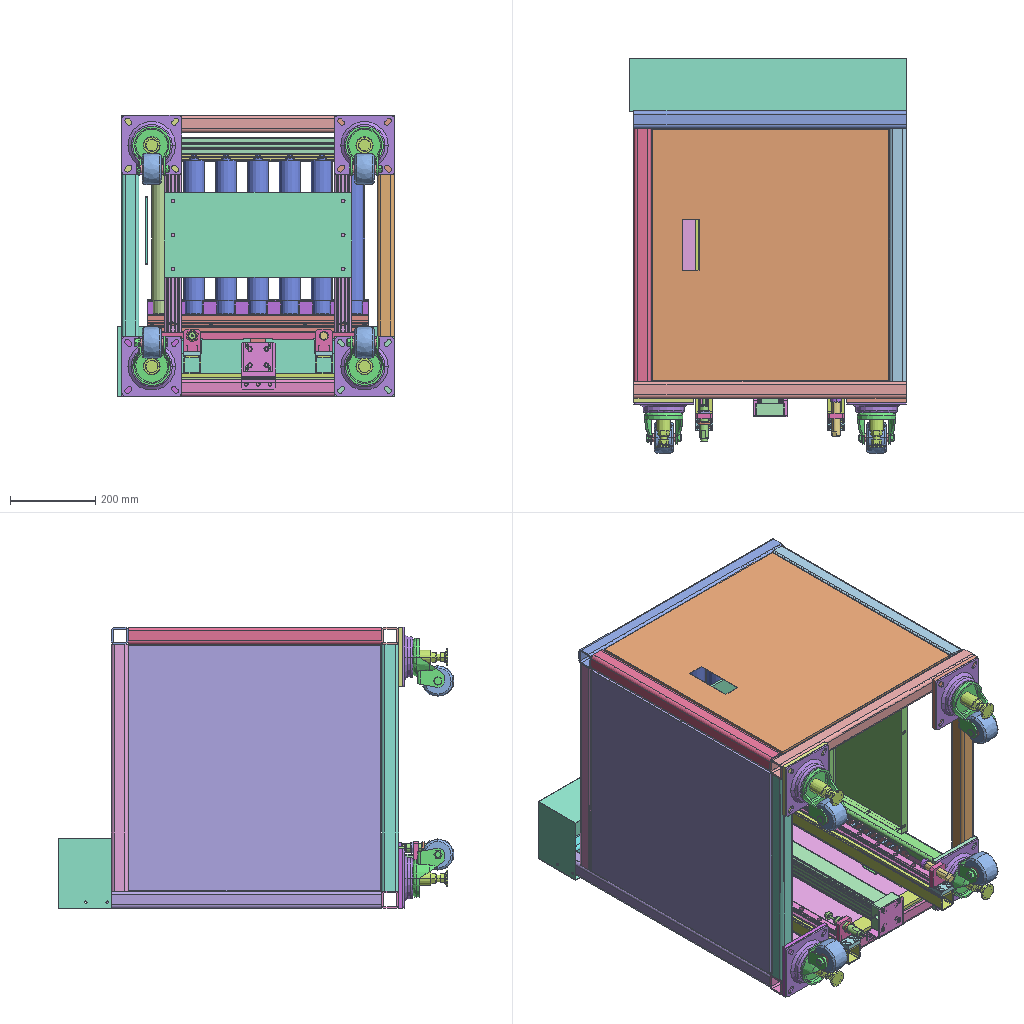Assembly | STEP file | 42 different items | 130 placed | box 652 x 930 x 661 mm
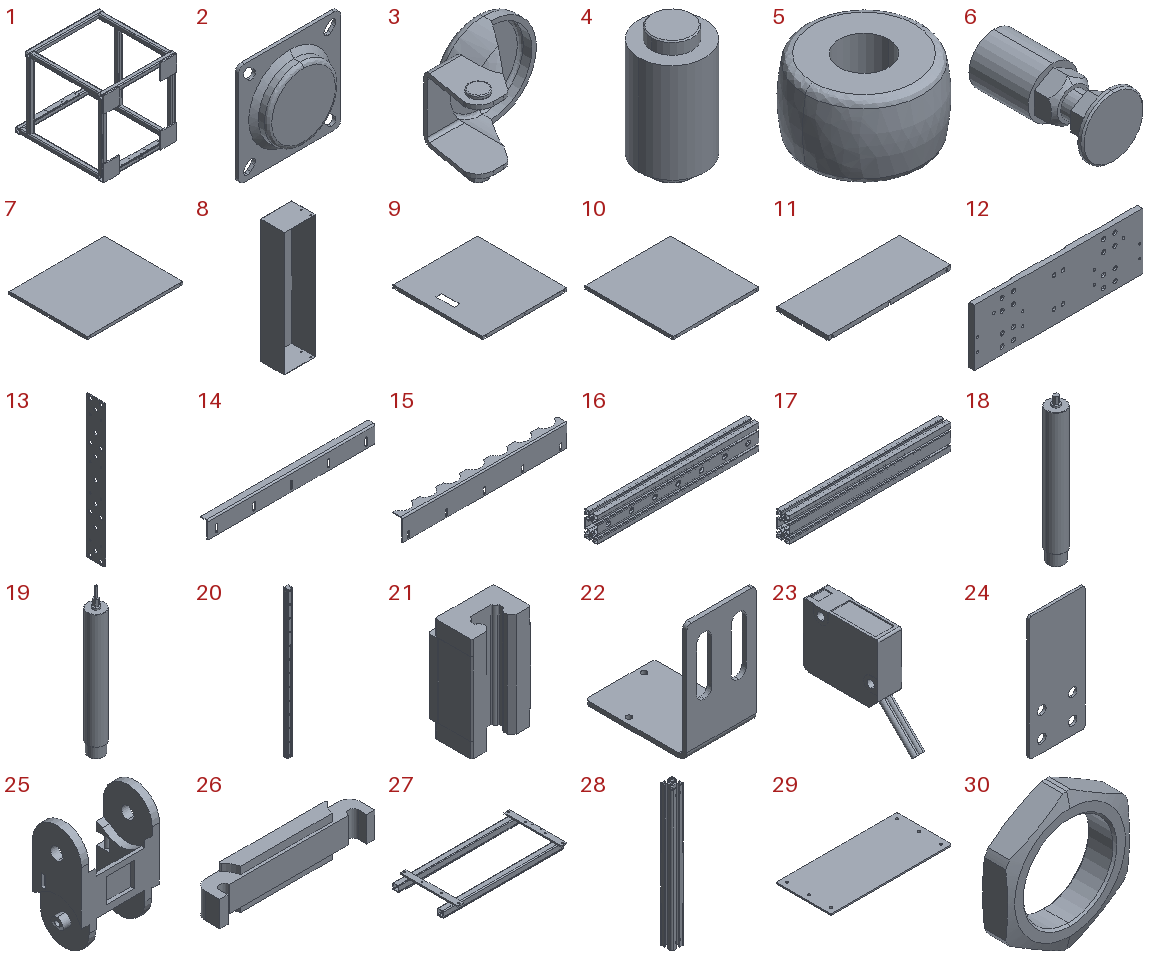Parts list (item | name | quantity | parent item | size | volume):
1 | - | x1 | - | 640 x 785 x 660 mm | 4940885 mm3
2 | CDAN75-Ms | x4 | in CDAN75-M | 140 x 23.5 x 140 mm | 226200 mm3
3 | CDAN75-Mb | x4 | in CDAN75-M | 116 x 74 x 90 mm | 70869 mm3
4 | CDAN75-Mbe | x4 | in CDAN75-M | 30 x 30 x 56 mm | 34751 mm3
5 | CDAN75-Mw | x4 | in CDAN75-M | 75 x 74.925 x 45 mm | 156321 mm3
6 | CDAN75-Ma | x4 | in CDAN75-M | 40 x 77 x 40 mm | 48272 mm3
7 | - | x1 | - | 683 x 558 x 20 mm | 427125 mm3
8 | - | x1 | - | 165 x 125 x 652 mm | 309587 mm3
9 | - | x1 | - | 558 x 593 x 20 mm | 368788 mm3
10 | - | x1 | - | 578 x 593 x 20 mm | 386105 mm3
11 | - | x1 | - | 578 x 240 x 20 mm | 168657 mm3
12 | - | x1 | - | 520 x 16 x 175 mm | 1376606 mm3
13 | - | x2 | - | 3 x 70 x 520 mm | 101913 mm3
14 | - | x1 | - | 470 x 20 x 48 mm | 59388 mm3
15 | - | x1 | - | 520 x 30 x 70 mm | 90245 mm3
16 | - | x1 | - | 520 x 40 x 80 mm | 382140 mm3
17 | - | x1 | - | 520 x 40 x 80 mm | 378549 mm3
18 | Unpowered roller_Default | x6 | - | 50.6 x 50.6 x 396 mm | 712589 mm3
19 | Electric roller_Default | x1 | - | 50.6 x 50.6 x 426 mm | 713178 mm3
20 | HGH25 rail | x2 | in HGH25CA2R740Z0 | 23 x 22 x 740 mm | 310065 mm3
21 | HGH25 slider | x4 | in HGH25CA2R740Z0 | 48 x 34.5 x 82 mm | 100220 mm3
22 | - | x1 | - | 32 x 47 x 55 mm | 5577 mm3
23 | Proximity switch | x1 | - | 10.4 x 45.161 x 39.591 mm | 8353 mm3
24 | - | x1 | - | 45 x 2 x 100 mm | 8685 mm3
25 | MHPU203_30c | x25 | in MHPU203_30_MHPU203-30 | 32 x 20 x 45 mm | 6087 mm3
26 | MHPU203_30f | x25 | in MHPU203_30_MHPU203-30 | 27.6 x 4.5 x 7.143 mm | 492.21 mm3
27 | - | x1 | - | 840 x 400 x 53 mm | 1080937 mm3
28 | - | x2 | - | 40 x 40 x 458 mm | 262404 mm3
29 | - | x1 | - | 440 x 200 x 5 mm | 437984 mm3
30 | ACA-2020-1 | x2 | in ACA-2020 | 26 x 6 x 29.132 mm | 1676 mm3
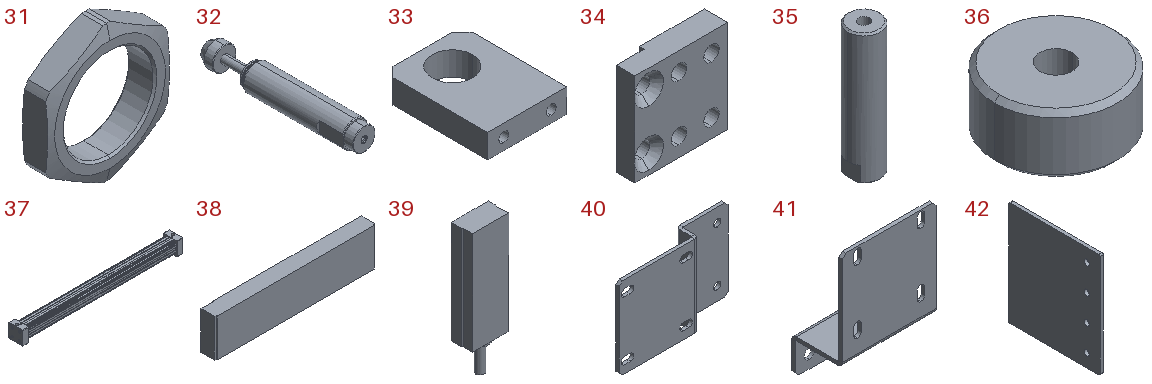31 | ACA-2020-2 | x2 | in ACA-2020 | 26 x 6 x 29.132 mm | 1676 mm3
32 | ACA-2020-3 | x2 | in ACA-2020 | 20 x 118 x 20 mm | 28972 mm3
33 | - | x5 | - | 40 x 53 x 12 mm | 20571 mm3
34 | - | x5 | - | 40 x 10 x 40 mm | 12395 mm3
35 | - | x2 | - | 20 x 20 x 80 mm | 24015 mm3
36 | - | x2 | - | 25 x 25 x 12 mm | 5014 mm3
37 | HI_PRU40500b | x1 | in PRF40x500-S2_0_ | 800 x 69 x 69 mm | 2639652 mm3
38 | HI_PRF40500s | x1 | in PRF40x500-S2_0_ | 152 x 14 x 36 mm | 74599 mm3
39 | HI_S-CS-95 | x2 | in PRF40x500-S2_0_ | 10.9 x 7 x 39 mm | 1983 mm3
40 | - | x1 | - | 115 x 18 x 75 mm | 27777 mm3
41 | - | x1 | - | 80 x 43 x 110 mm | 34046 mm3
42 | - | x1 | - | 5 x 140 x 160 mm | 110710 mm3
Placements (level | parent | child | x y z in mm | rotation matrix by rows):
1 | subassembly 2 | subassembly 3 | -327.676 8.356 -0.0 | 1 0 0 0 1 0 0 0 1
2 | subassembly 3 | subassembly 4 | -159.675 -6.067 -330.0 | 1 0 0 0 1 0 0 0 1
2 | subassembly 3 | CDAN75-M | -409.675 -422.067 240.0 | 0 0 -1 0 1 0 1 0 0
3 | CDAN75-M | CDAN75-Ms | -0.0 -0.0 -0.0 | 1 0 0 0 1 0 0 0 1
3 | CDAN75-M | CDAN75-Mb | -0.0 -0.0 -0.0 | 1 0 0 0 1 0 0 0 1
3 | CDAN75-M | CDAN75-Mbe | -0.0 -0.0 -0.0 | 1 0 0 0 1 0 0 0 1
3 | CDAN75-M | CDAN75-Mw | -0.0 -0.0 -0.0 | 1 0 0 0 1 0 0 0 1
3 | CDAN75-M | CDAN75-Ma | -0.0 -0.0 -0.0 | 1 0 0 0 1 0 0 0 1
2 | subassembly 3 | CDAN75-M | 90.325 -422.067 240.0 | 0 0 -1 0 1 0 1 0 0
3 | CDAN75-M | CDAN75-Ms | -0.0 -0.0 -0.0 | 1 0 0 0 1 0 0 0 1
3 | CDAN75-M | CDAN75-Mb | -0.0 -0.0 -0.0 | 1 0 0 0 1 0 0 0 1
3 | CDAN75-M | CDAN75-Mbe | -0.0 -0.0 -0.0 | 1 0 0 0 1 0 0 0 1
3 | CDAN75-M | CDAN75-Mw | -0.0 -0.0 -0.0 | 1 0 0 0 1 0 0 0 1
3 | CDAN75-M | CDAN75-Ma | -0.0 -0.0 -0.0 | 1 0 0 0 1 0 0 0 1
2 | subassembly 3 | CDAN75-M | -409.675 -422.067 -280.0 | 0 0 1 0 1 0 -1 0 0
3 | CDAN75-M | CDAN75-Ms | -0.0 -0.0 -0.0 | 1 0 0 0 1 0 0 0 1
3 | CDAN75-M | CDAN75-Mb | -0.0 -0.0 -0.0 | 1 0 0 0 1 0 0 0 1
3 | CDAN75-M | CDAN75-Mbe | -0.0 -0.0 -0.0 | 1 0 0 0 1 0 0 0 1
3 | CDAN75-M | CDAN75-Mw | -0.0 -0.0 -0.0 | 1 0 0 0 1 0 0 0 1
3 | CDAN75-M | CDAN75-Ma | -0.0 -0.0 -0.0 | 1 0 0 0 1 0 0 0 1
2 | subassembly 3 | CDAN75-M | 90.325 -422.067 -280.0 | 0 0 1 0 1 0 -1 0 0
3 | CDAN75-M | CDAN75-Ms | -0.0 -0.0 -0.0 | 1 0 0 0 1 0 0 0 1
3 | CDAN75-M | CDAN75-Mb | -0.0 -0.0 -0.0 | 1 0 0 0 1 0 0 0 1
3 | CDAN75-M | CDAN75-Mbe | -0.0 -0.0 -0.0 | 1 0 0 0 1 0 0 0 1
3 | CDAN75-M | CDAN75-Mw | -0.0 -0.0 -0.0 | 1 0 0 0 1 0 0 0 1
3 | CDAN75-M | CDAN75-Ma | -0.0 -0.0 -0.0 | 1 0 0 0 1 0 0 0 1
2 | subassembly 3 | subassembly 5 | 118.325 334.433 -330.0 | 0 -1 0 -1 0 0 0 0 -1
2 | subassembly 3 | subassembly 6 | -490.675 -398.567 -351.0 | 0 0 1 0 1 0 -1 0 0
2 | subassembly 3 | subassembly 7 | -437.675 -348.567 290.0 | 1 0 0 0 1 0 0 0 1
2 | subassembly 3 | subassembly 8 | -459.675 -346.567 -310.0 | 0 0 -1 0 1 0 1 0 -0
2 | subassembly 3 | subassembly 9 | 140.325 73.933 -308.0 | 0 0 1 0 -1 0 1 0 0
1 | subassembly 2 | subassembly 10 | -407.188 173.195 -347.955 | 0 0 1 0 1 0 -1 0 0
2 | subassembly 10 | subassembly 11 | -147.955 36.01 -80.412 | 0 1 0 0 0 -1 -1 0 0
2 | subassembly 10 | subassembly 12 | -187.955 71.51 -340.412 | -1 0 0 0 1 0 0 0 -1
2 | subassembly 10 | subassembly 12 | -558.455 71.51 -340.412 | -1 0 0 0 1 0 0 0 -1
2 | subassembly 10 | subassembly 13 | -598.455 98.51 129.588 | 0 0 1 0 1 0 -1 0 -0
2 | subassembly 10 | subassembly 14 | -154.455 100.51 179.588 | 0 0 -1 0 -1 0 -1 0 0
2 | subassembly 10 | subassembly 15 | -585.955 78.51 -340.412 | 0 1 0 0 0 1 1 0 0
2 | subassembly 10 | subassembly 16 | -167.955 38.51 -340.412 | 0 -1 0 0 0 -1 1 0 0
2 | subassembly 10 | Unpowered roller_Default | -222.455 58.76 -230.412 | 0 0 -1 0.3439 -0.939 0 -0.939 -0.3439 0
2 | subassembly 10 | Unpowered roller_Default | -222.455 58.76 144.588 | 0 0 -1 0.3439 -0.939 0 -0.939 -0.3439 0
2 | subassembly 10 | Unpowered roller_Default | -222.455 58.76 69.588 | 0 0 -1 0.3439 -0.939 0 -0.939 -0.3439 0
2 | subassembly 10 | Unpowered roller_Default | -222.455 58.76 -5.412 | 0 0 -1 0.3439 -0.939 0 -0.939 -0.3439 0
2 | subassembly 10 | Unpowered roller_Default | -222.455 58.76 -80.412 | 0 0 -1 0.3439 -0.939 0 -0.939 -0.3439 0
2 | subassembly 10 | Unpowered roller_Default | -222.455 58.76 -155.412 | 0 0 -1 0.3439 -0.939 0 -0.939 -0.3439 0
2 | subassembly 10 | Electric roller_Default | -222.455 58.361 -305.412 | 0 0 -1 0 1 0 1 0 0
2 | subassembly 10 | HGH25CA2R740Z0 | -108.387 -214.405 -232.617 | 0 -1 0 0 0 1 -1 0 -0
3 | HGH25CA2R740Z0 | HGH25 rail | 4.046 -14.432 -225.0 | 1 0 0 0 1 0 0 0 1
3 | HGH25CA2R740Z0 | HGH25 slider | 4.046 -14.432 297.916 | 1 0 0 0 1 0 0 0 1
3 | HGH25CA2R740Z0 | HGH25 slider | 4.046 -14.432 202.916 | 1 0 0 0 1 0 0 0 1
2 | subassembly 10 | HGH25CA2R740Z0 | -108.387 -214.405 80.383 | 0 -1 0 0 0 1 -1 0 -0
3 | HGH25CA2R740Z0 | HGH25 rail | 4.046 -14.432 -225.0 | 1 0 0 0 1 0 0 0 1
3 | HGH25CA2R740Z0 | HGH25 slider | 4.046 -14.432 297.916 | 1 0 0 0 1 0 0 0 1
3 | HGH25CA2R740Z0 | HGH25 slider | 4.046 -14.432 202.916 | 1 0 0 0 1 0 0 0 1
2 | subassembly 10 | subassembly 17 | -605.955 115.71 169.588 | 0 1 0 0 0 -1 -1 0 -0
2 | subassembly 10 | Proximity switch | -563.955 108.51 145.388 | 0 0 1 -1 0 0 0 -1 0
2 | subassembly 10 | subassembly 18 | -47.955 -410.405 53.338 | 0 -1 0 1 0 0 0 0 1
2 | subassembly 10 | MHPU203_30_MHPU203-30 | -119.955 58.095 139.338 | 0 1 0 -1 0 0 0 0 1
3 | MHPU203_30_MHPU203-30 | MHPU203_30c | 32.5 0.0 -0.0 | 0 0 1 0 1 0 -1 0 -0
3 | MHPU203_30_MHPU203-30 | MHPU203_30f | 10.0 0.0 -0.0 | 0 0 1 0 1 0 -1 0 -0
3 | MHPU203_30_MHPU203-30 | MHPU203_30c | 7.067 -2.909 -0.0 | 0 0.2909 0.9567 0 0.9567 -0.2909 -1 0 0
3 | MHPU203_30_MHPU203-30 | MHPU203_30f | -14.459 3.637 -0.0 | 0 0.2909 0.9567 0 0.9567 -0.2909 -1 0 0
3 | MHPU203_30_MHPU203-30 | MHPU203_30c | -22.252 -1.817 -0.0 | 0 0.9091 0.4167 0 0.4167 -0.9091 -1 0 0
3 | MHPU203_30_MHPU203-30 | MHPU203_30f | -31.627 18.637 -0.0 | 0 0.9091 0.4167 0 0.4167 -0.9091 -1 0 0
3 | MHPU203_30_MHPU203-30 | MHPU203_30c | -41.002 20.909 -0.0 | 0 0.9091 -0.4167 0 -0.4167 -0.9091 -1 0 0
3 | MHPU203_30_MHPU203-30 | MHPU203_30f | -31.627 41.363 -0.0 | 0 0.9091 -0.4167 0 -0.4167 -0.9091 -1 0 0
3 | MHPU203_30_MHPU203-30 | MHPU203_30c | -35.986 49.817 -0.0 | 0 0.2909 -0.9567 0 -0.9567 -0.2909 -1 0 0
3 | MHPU203_30_MHPU203-30 | MHPU203_30f | -14.459 56.363 -0.0 | 0 0.2909 -0.9567 0 -0.9567 -0.2909 -1 0 0
3 | MHPU203_30_MHPU203-30 | MHPU203_30c | -12.5 60.0 -0.0 | 0 0 -1 0 -1 0 -1 0 0
3 | MHPU203_30_MHPU203-30 | MHPU203_30f | 10 60.0 -0.0 | 0 0 -1 0 -1 0 -1 0 0
3 | MHPU203_30_MHPU203-30 | MHPU203_30c | 12.5 60.0 -0.0 | 0 0 -1 0 -1 0 -1 0 0
3 | MHPU203_30_MHPU203-30 | MHPU203_30f | 35 60.0 -0.0 | 0 0 -1 0 -1 0 -1 0 0
3 | MHPU203_30_MHPU203-30 | MHPU203_30c | 37.5 60.0 -0.0 | 0 0 -1 0 -1 0 -1 0 0
3 | MHPU203_30_MHPU203-30 | MHPU203_30f | 60 60.0 -0.0 | 0 0 -1 0 -1 0 -1 0 0
3 | MHPU203_30_MHPU203-30 | MHPU203_30c | 62.5 60.0 -0.0 | 0 0 -1 0 -1 0 -1 0 0
3 | MHPU203_30_MHPU203-30 | MHPU203_30f | 85 60.0 -0.0 | 0 0 -1 0 -1 0 -1 0 0
3 | MHPU203_30_MHPU203-30 | MHPU203_30c | 87.5 60.0 -0.0 | 0 0 -1 0 -1 0 -1 0 0
3 | MHPU203_30_MHPU203-30 | MHPU203_30f | 110 60.0 -0.0 | 0 0 -1 0 -1 0 -1 0 0
3 | MHPU203_30_MHPU203-30 | MHPU203_30f | 135 60.0 -0.0 | 0 0 -1 0 -1 0 -1 0 0
3 | MHPU203_30_MHPU203-30 | MHPU203_30f | 160 60.0 -0.0 | 0 0 -1 0 -1 0 -1 0 0
3 | MHPU203_30_MHPU203-30 | MHPU203_30f | 185 60.0 -0.0 | 0 0 -1 0 -1 0 -1 0 0
3 | MHPU203_30_MHPU203-30 | MHPU203_30f | 210 60.0 -0.0 | 0 0 -1 0 -1 0 -1 0 0
3 | MHPU203_30_MHPU203-30 | MHPU203_30f | 235 60.0 -0.0 | 0 0 -1 0 -1 0 -1 0 0
3 | MHPU203_30_MHPU203-30 | MHPU203_30f | 260 60.0 -0.0 | 0 0 -1 0 -1 0 -1 0 0
3 | MHPU203_30_MHPU203-30 | MHPU203_30f | 285 60.0 -0.0 | 0 0 -1 0 -1 0 -1 0 0
3 | MHPU203_30_MHPU203-30 | MHPU203_30f | 310 60.0 -0.0 | 0 0 -1 0 -1 0 -1 0 0
3 | MHPU203_30_MHPU203-30 | MHPU203_30f | 335 60.0 -0.0 | 0 0 -1 0 -1 0 -1 0 0
3 | MHPU203_30_MHPU203-30 | MHPU203_30c | 112.5 60.0 -0.0 | 0 0 -1 0 -1 0 -1 0 0
3 | MHPU203_30_MHPU203-30 | MHPU203_30c | 137.5 60.0 -0.0 | 0 0 -1 0 -1 0 -1 0 0
3 | MHPU203_30_MHPU203-30 | MHPU203_30c | 162.5 60.0 -0.0 | 0 0 -1 0 -1 0 -1 0 0
3 | MHPU203_30_MHPU203-30 | MHPU203_30c | 187.5 60.0 -0.0 | 0 0 -1 0 -1 0 -1 0 0
3 | MHPU203_30_MHPU203-30 | MHPU203_30c | 212.5 60.0 -0.0 | 0 0 -1 0 -1 0 -1 0 0
3 | MHPU203_30_MHPU203-30 | MHPU203_30c | 237.5 60.0 -0.0 | 0 0 -1 0 -1 0 -1 0 0
3 | MHPU203_30_MHPU203-30 | MHPU203_30c | 262.5 60.0 -0.0 | 0 0 -1 0 -1 0 -1 0 0
3 | MHPU203_30_MHPU203-30 | MHPU203_30c | 287.5 60.0 -0.0 | 0 0 -1 0 -1 0 -1 0 0
3 | MHPU203_30_MHPU203-30 | MHPU203_30c | 312.5 60.0 -0.0 | 0 0 -1 0 -1 0 -1 0 0
3 | MHPU203_30_MHPU203-30 | MHPU203_30c | 57.5 0.0 -0.0 | 0 0 1 0 1 0 -1 0 -0
3 | MHPU203_30_MHPU203-30 | MHPU203_30f | 35.0 0.0 -0.0 | 0 0 1 0 1 0 -1 0 -0
3 | MHPU203_30_MHPU203-30 | MHPU203_30c | 337.5 60.0 -0.0 | 0 0 -1 0 -1 0 -1 0 0
3 | MHPU203_30_MHPU203-30 | MHPU203_30c | 362.5 60.0 -0.0 | 0 0 -1 0 -1 0 -1 0 0
3 | MHPU203_30_MHPU203-30 | MHPU203_30c | 387.5 60.0 -0.0 | 0 0 -1 0 -1 0 -1 0 0
3 | MHPU203_30_MHPU203-30 | MHPU203_30c | 412.5 60.0 -0.0 | 0 0 -1 0 -1 0 -1 0 0
3 | MHPU203_30_MHPU203-30 | MHPU203_30c | 437.5 60.0 -0.0 | 0 0 -1 0 -1 0 -1 0 0
3 | MHPU203_30_MHPU203-30 | MHPU203_30f | 360 60.0 -0.0 | 0 0 -1 0 -1 0 -1 0 0
3 | MHPU203_30_MHPU203-30 | MHPU203_30f | 385 60.0 -0.0 | 0 0 -1 0 -1 0 -1 0 0
3 | MHPU203_30_MHPU203-30 | MHPU203_30f | 410 60.0 -0.0 | 0 0 -1 0 -1 0 -1 0 0
3 | MHPU203_30_MHPU203-30 | MHPU203_30f | 435 60.0 -0.0 | 0 0 -1 0 -1 0 -1 0 0
3 | MHPU203_30_MHPU203-30 | MHPU203_30f | 460 60.0 -0.0 | 0 0 -1 0 -1 0 -1 0 0
2 | subassembly 10 | subassembly 19 | -70.955 -628.405 -235.162 | 0 0 1 1 0 0 0 1 -0
2 | subassembly 10 | subassembly 20 | -147.955 -1.49 -280.412 | 0 0 1 0 1 0 -1 0 -0
2 | subassembly 10 | subassembly 20 | -147.955 -1.49 119.588 | 0 0 1 0 1 0 -1 0 -0
2 | subassembly 10 | subassembly 21 | -476.955 -26.49 -300.412 | 0 1 0 0 0 1 1 0 -0
2 | subassembly 10 | ACA-2020 | -139.955 -653.405 -235.162 | -0.9745 0 0.2243 0 1 0 -0.2243 0 -0.9745
3 | ACA-2020 | ACA-2020-1 | 0.0 -22.0 -0.0 | 0.9939 0 -0.11 0 1 0 0.11 0 0.9939
3 | ACA-2020 | ACA-2020-2 | 0.0 -2.0 0.0 | 0.9756 0 0.2198 0 1 0 -0.2198 0 0.9756
3 | ACA-2020 | ACA-2020-3 | 0.0 0.0 -0.0 | 1 0 0 0 1 0 0 0 1
2 | subassembly 10 | subassembly 22 | -101.955 -588.405 -255.162 | 0 -1 0 0 0 -1 1 0 -0
2 | subassembly 10 | subassembly 23 | -93.955 -588.405 -215.162 | 0 -1 0 -1 0 0 0 0 -1
2 | subassembly 10 | subassembly 23 | -93.955 171.595 -255.162 | 0 -1 0 1 0 0 0 0 1
2 | subassembly 10 | subassembly 22 | -101.955 183.595 -255.162 | 0 -1 0 0 0 -1 1 0 0
2 | subassembly 10 | ACA-2020 | -139.955 228.595 -235.162 | 0.9385 0 0.3453 0 -1 0 0.3453 0 -0.9385
3 | ACA-2020 | ACA-2020-1 | 0.0 -22.0 -0.0 | 0.9939 0 -0.11 0 1 0 0.11 0 0.9939
3 | ACA-2020 | ACA-2020-2 | 0.0 -2.0 0.0 | 0.9756 0 0.2198 0 1 0 -0.2198 0 0.9756
3 | ACA-2020 | ACA-2020-3 | 0.0 0.0 -0.0 | 1 0 0 0 1 0 0 0 1
2 | subassembly 10 | subassembly 23 | -93.955 171.595 54.838 | 0 -1 0 1 0 0 0 0 1
2 | subassembly 10 | subassembly 22 | -101.955 183.595 54.838 | 0 -1 0 0 0 -1 1 0 0
2 | subassembly 10 | subassembly 24 | -139.955 234.595 74.838 | 1 0 0 0 0 -1 0 1 -0
2 | subassembly 10 | subassembly 24 | -139.955 -641.405 74.838 | 0.8372 0.5469 0 0 0 1 0.5469 -0.8372 -0
2 | subassembly 10 | subassembly 25 | -139.955 142.595 74.838 | 0.9237 0.383 0 0 0 1 0.383 -0.9237 0
2 | subassembly 10 | subassembly 25 | -139.955 -549.405 74.838 | 1 0 0 0 0 -1 0 1 0
2 | subassembly 10 | subassembly 22 | -101.955 -588.405 54.838 | 0 -1 0 0 0 -1 1 0 -0
2 | subassembly 10 | subassembly 23 | -93.955 -588.405 94.838 | 0 -1 0 -1 0 0 0 0 -1
2 | subassembly 10 | subassembly 23 | -93.955 171.595 54.838 | 0 -1 0 1 0 0 0 0 1
2 | subassembly 10 | subassembly 22 | -101.955 183.595 54.838 | 0 -1 0 0 0 -1 1 0 0
2 | subassembly 10 | PRF40x500-S2_0_ | -61.701 185.013 -59.225 | 0 -1 0 0 0 1 -1 0 0
3 | PRF40x500-S2_0_ | HI_PRU40500b | 20.938 -6.247 21.581 | 0 0 1 0 1 0 -1 0 0
3 | PRF40x500-S2_0_ | HI_PRF40500s | 20.938 58.253 -149.003 | 0 0 -1 0 1 0 1 0 -0
3 | PRF40x500-S2_0_ | HI_S-CS-95 | 28.1 35.4 -2.5 | 0 1 0 -1 0 0 0 0 1
3 | PRF40x500-S2_0_ | HI_S-CS-95 | 28.1 35.4 -741.5 | 0 1 0 1 0 0 0 0 -1
2 | subassembly 10 | subassembly 26 | -124.455 209.595 -117.662 | 1 0 0 0 1 0 0 0 1
2 | subassembly 10 | subassembly 27 | -124.455 -593.405 -120.162 | 0 0 -1 0 1 0 1 0 0
2 | subassembly 10 | subassembly 28 | -467.455 -21.339 -340.412 | 0 0 1 0 1 0 -1 0 -0